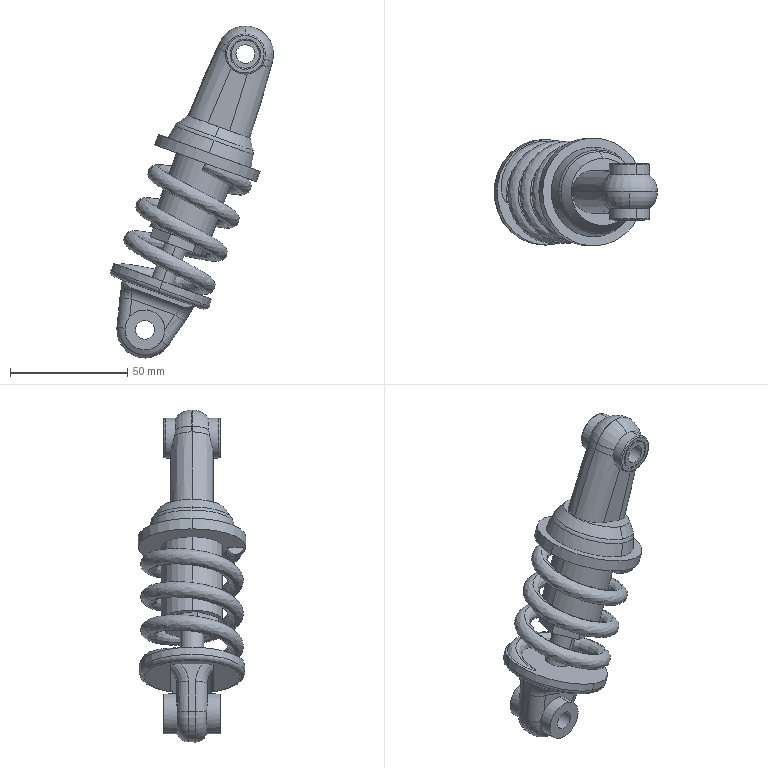Part | SolidWorks | features BaseBody 1 | 1 solid | 99 faces | box 69.615 x 46 x 141.456 mm | volume 89159 mm3 | cylinder 33 | plane 26 | torus 22 | spline 14 | cone 4 | commonest cylinder face diameters 17 x8 8 x4 10 x4 12 x4 24 x3 26.217 x2